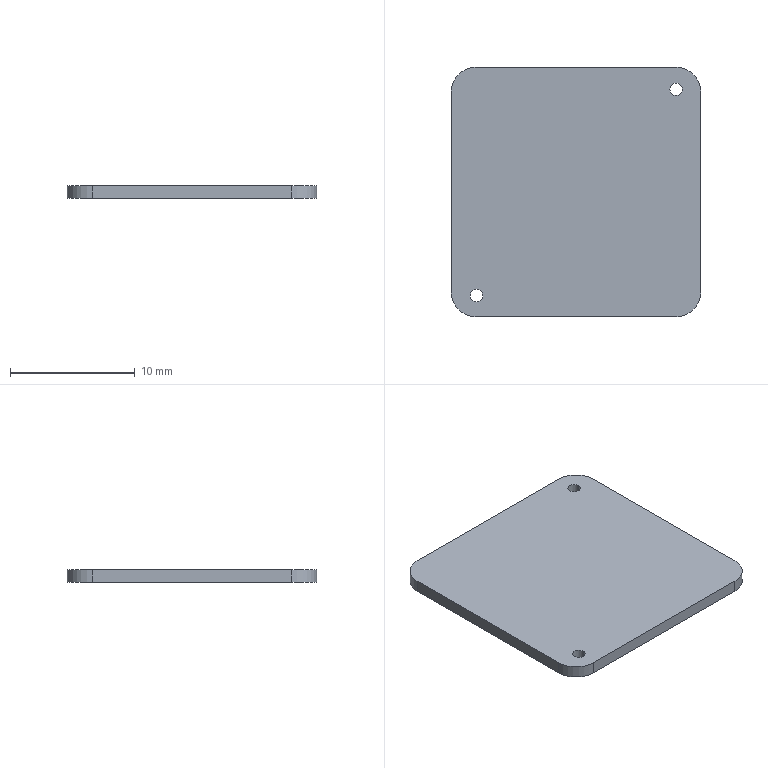Part | SolidWorks | features Extrusion 1, Fillet 1, ICE 1 | 1 solid | 14 faces | box 20 x 20 x 1 mm | volume 394.996 mm3 | cylinder 8 | plane 6 | commonest cylinder face diameters 1 x4 4 x4
STEP:
#1=CARTESIAN_POINT('',(-8.473,-8.297,0.));
#2=VERTEX_POINT('',#1);
#3=CARTESIAN_POINT('',(-7.473,-8.297,0.));
#4=VERTEX_POINT('',#3);
#5=CARTESIAN_POINT('',(-7.973,-8.297,0.));
#6=DIRECTION('',(0.,0.,1.));
#7=DIRECTION('',(1.,0.,0.));
#8=AXIS2_PLACEMENT_3D('',#5,#6,#7);
#9=CIRCLE('',#8,0.5);
#10=EDGE_CURVE('',#2,#4,#9,.T.);
#11=ORIENTED_EDGE('',*,*,#10,.F.);
#12=CARTESIAN_POINT('',(-8.473,-8.297,1.));
#13=VERTEX_POINT('',#12);
#14=CARTESIAN_POINT('',(-8.473,-8.297,0.));
#15=DIRECTION('',(0.,0.,1.));
#16=VECTOR('',#15,1000.);
#17=LINE('',#14,#16);
#18=EDGE_CURVE('',#2,#13,#17,.T.);
#19=ORIENTED_EDGE('',*,*,#18,.T.);
#20=CARTESIAN_POINT('',(-7.473,-8.297,1.));
#21=VERTEX_POINT('',#20);
#22=CARTESIAN_POINT('',(-7.973,-8.297,1.));
#23=DIRECTION('',(0.,0.,1.));
#24=DIRECTION('',(1.,0.,0.));
#25=AXIS2_PLACEMENT_3D('',#22,#23,#24);
#26=CIRCLE('',#25,0.5);
#27=EDGE_CURVE('',#13,#21,#26,.T.);
#28=ORIENTED_EDGE('',*,*,#27,.T.);
#29=CARTESIAN_POINT('',(-7.473,-8.297,0.));
#30=DIRECTION('',(0.,0.,1.));
#31=VECTOR('',#30,1000.);
#32=LINE('',#29,#31);
#33=EDGE_CURVE('',#4,#21,#32,.T.);
#34=ORIENTED_EDGE('',*,*,#33,.F.);
#35=EDGE_LOOP('',(#11,#19,#28,#34));
#36=FACE_OUTER_BOUND('',#35,.T.);
#37=CARTESIAN_POINT('',(-7.973,-8.297,0.));
#38=DIRECTION('',(0.,0.,1.));
#39=DIRECTION('',(1.,0.,0.));
#40=AXIS2_PLACEMENT_3D('',#37,#38,#39);
#41=CYLINDRICAL_SURFACE('',#40,0.5);
#42=ADVANCED_FACE('',(#36),#41,.F.);
#43=CARTESIAN_POINT('',(7.521,8.23,0.));
#44=VERTEX_POINT('',#43);
#45=CARTESIAN_POINT('',(8.521,8.23,0.));
#46=VERTEX_POINT('',#45);
#47=CARTESIAN_POINT('',(8.021,8.23,0.));
#48=DIRECTION('',(0.,0.,1.));
#49=DIRECTION('',(1.,0.,0.));
#50=AXIS2_PLACEMENT_3D('',#47,#48,#49);
#51=CIRCLE('',#50,0.5);
#52=EDGE_CURVE('',#44,#46,#51,.T.);
#53=ORIENTED_EDGE('',*,*,#52,.F.);
#54=CARTESIAN_POINT('',(7.521,8.23,1.));
#55=VERTEX_POINT('',#54);
#56=CARTESIAN_POINT('',(7.521,8.23,0.));
#57=DIRECTION('',(0.,0.,1.));
#58=VECTOR('',#57,1000.);
#59=LINE('',#56,#58);
#60=EDGE_CURVE('',#44,#55,#59,.T.);
#61=ORIENTED_EDGE('',*,*,#60,.T.);
#62=CARTESIAN_POINT('',(8.521,8.23,1.));
#63=VERTEX_POINT('',#62);
#64=CARTESIAN_POINT('',(8.021,8.23,1.));
#65=DIRECTION('',(0.,0.,1.));
#66=DIRECTION('',(1.,0.,0.));
#67=AXIS2_PLACEMENT_3D('',#64,#65,#66);
#68=CIRCLE('',#67,0.5);
#69=EDGE_CURVE('',#55,#63,#68,.T.);
#70=ORIENTED_EDGE('',*,*,#69,.T.);
#71=CARTESIAN_POINT('',(8.521,8.23,0.));
#72=DIRECTION('',(0.,0.,1.));
#73=VECTOR('',#72,1000.);
#74=LINE('',#71,#73);
#75=EDGE_CURVE('',#46,#63,#74,.T.);
#76=ORIENTED_EDGE('',*,*,#75,.F.);
#77=EDGE_LOOP('',(#53,#61,#70,#76));
#78=FACE_OUTER_BOUND('',#77,.T.);
#79=CARTESIAN_POINT('',(8.021,8.23,0.));
#80=DIRECTION('',(0.,0.,1.));
#81=DIRECTION('',(1.,0.,0.));
#82=AXIS2_PLACEMENT_3D('',#79,#80,#81);
#83=CYLINDRICAL_SURFACE('',#82,0.5);
#84=ADVANCED_FACE('',(#78),#83,.F.);
#85=CARTESIAN_POINT('',(10.,-8.,0.));
#86=VERTEX_POINT('',#85);
#87=CARTESIAN_POINT('',(10.,8.,0.));
#88=VERTEX_POINT('',#87);
#89=CARTESIAN_POINT('',(10.,10.,0.));
#90=DIRECTION('',(0.,1.,0.));
#91=VECTOR('',#90,1000.);
#92=LINE('',#89,#91);
#93=EDGE_CURVE('',#86,#88,#92,.T.);
#94=ORIENTED_EDGE('',*,*,#93,.T.);
#95=CARTESIAN_POINT('',(10.,8.,1.));
#96=VERTEX_POINT('',#95);
#97=CARTESIAN_POINT('',(10.,8.,1.));
#98=DIRECTION('',(0.,0.,1.));
#99=VECTOR('',#98,1000.);
#100=LINE('',#97,#99);
#101=EDGE_CURVE('',#88,#96,#100,.T.);
#102=ORIENTED_EDGE('',*,*,#101,.T.);
#103=CARTESIAN_POINT('',(10.,-8.,1.));
#104=VERTEX_POINT('',#103);
#105=CARTESIAN_POINT('',(10.,10.,1.));
#106=DIRECTION('',(0.,1.,0.));
#107=VECTOR('',#106,1000.);
#108=LINE('',#105,#107);
#109=EDGE_CURVE('',#104,#96,#108,.T.);
#110=ORIENTED_EDGE('',*,*,#109,.F.);
#111=CARTESIAN_POINT('',(10.,-8.,1.));
#112=DIRECTION('',(0.,0.,-1.));
#113=VECTOR('',#112,1000.);
#114=LINE('',#111,#113);
#115=EDGE_CURVE('',#104,#86,#114,.T.);
#116=ORIENTED_EDGE('',*,*,#115,.T.);
#117=EDGE_LOOP('',(#94,#102,#110,#116));
#118=FACE_OUTER_BOUND('',#117,.T.);
#119=CARTESIAN_POINT('',(10.,10.,1.));
#120=DIRECTION('',(-1.,0.,0.));
#121=DIRECTION('',(0.,0.,1.));
#122=AXIS2_PLACEMENT_3D('',#119,#120,#121);
#123=PLANE('',#122);
#124=ADVANCED_FACE('',(#118),#123,.F.);
#125=CARTESIAN_POINT('',(8.,10.,1.));
#126=VERTEX_POINT('',#125);
#127=CARTESIAN_POINT('',(-8.,10.,1.));
#128=VERTEX_POINT('',#127);
#129=CARTESIAN_POINT('',(-10.,10.,1.));
#130=DIRECTION('',(-1.,0.,0.));
#131=VECTOR('',#130,1000.);
#132=LINE('',#129,#131);
#133=EDGE_CURVE('',#126,#128,#132,.T.);
#134=ORIENTED_EDGE('',*,*,#133,.F.);
#135=CARTESIAN_POINT('',(8.,10.,0.));
#136=VERTEX_POINT('',#135);
#137=CARTESIAN_POINT('',(8.,10.,1.));
#138=DIRECTION('',(0.,0.,-1.));
#139=VECTOR('',#138,1000.);
#140=LINE('',#137,#139);
#141=EDGE_CURVE('',#126,#136,#140,.T.);
#142=ORIENTED_EDGE('',*,*,#141,.T.);
#143=CARTESIAN_POINT('',(-8.,10.,0.));
#144=VERTEX_POINT('',#143);
#145=CARTESIAN_POINT('',(-10.,10.,0.));
#146=DIRECTION('',(-1.,0.,0.));
#147=VECTOR('',#146,1000.);
#148=LINE('',#145,#147);
#149=EDGE_CURVE('',#136,#144,#148,.T.);
#150=ORIENTED_EDGE('',*,*,#149,.T.);
#151=CARTESIAN_POINT('',(-8.,10.,1.));
#152=DIRECTION('',(0.,0.,1.));
#153=VECTOR('',#152,1000.);
#154=LINE('',#151,#153);
#155=EDGE_CURVE('',#144,#128,#154,.T.);
#156=ORIENTED_EDGE('',*,*,#155,.T.);
#157=EDGE_LOOP('',(#134,#142,#150,#156));
#158=FACE_OUTER_BOUND('',#157,.T.);
#159=CARTESIAN_POINT('',(-10.,10.,1.));
#160=DIRECTION('',(0.,-1.,0.));
#161=DIRECTION('',(0.,0.,-1.));
#162=AXIS2_PLACEMENT_3D('',#159,#160,#161);
#163=PLANE('',#162);
#164=ADVANCED_FACE('',(#158),#163,.F.);
#165=CARTESIAN_POINT('',(-10.,8.,0.));
#166=VERTEX_POINT('',#165);
#167=CARTESIAN_POINT('',(-10.,-8.,0.));
#168=VERTEX_POINT('',#167);
#169=CARTESIAN_POINT('',(-10.,10.,0.));
#170=DIRECTION('',(0.,-1.,0.));
#171=VECTOR('',#170,1000.);
#172=LINE('',#169,#171);
#173=EDGE_CURVE('',#166,#168,#172,.T.);
#174=ORIENTED_EDGE('',*,*,#173,.T.);
#175=CARTESIAN_POINT('',(-10.,-8.,1.));
#176=VERTEX_POINT('',#175);
#177=CARTESIAN_POINT('',(-10.,-8.,1.));
#178=DIRECTION('',(0.,0.,1.));
#179=VECTOR('',#178,1000.);
#180=LINE('',#177,#179);
#181=EDGE_CURVE('',#168,#176,#180,.T.);
#182=ORIENTED_EDGE('',*,*,#181,.T.);
#183=CARTESIAN_POINT('',(-10.,8.,1.));
#184=VERTEX_POINT('',#183);
#185=CARTESIAN_POINT('',(-10.,10.,1.));
#186=DIRECTION('',(0.,-1.,0.));
#187=VECTOR('',#186,1000.);
#188=LINE('',#185,#187);
#189=EDGE_CURVE('',#184,#176,#188,.T.);
#190=ORIENTED_EDGE('',*,*,#189,.F.);
#191=CARTESIAN_POINT('',(-10.,8.,1.));
#192=DIRECTION('',(0.,0.,-1.));
#193=VECTOR('',#192,1000.);
#194=LINE('',#191,#193);
#195=EDGE_CURVE('',#184,#166,#194,.T.);
#196=ORIENTED_EDGE('',*,*,#195,.T.);
#197=EDGE_LOOP('',(#174,#182,#190,#196));
#198=FACE_OUTER_BOUND('',#197,.T.);
#199=CARTESIAN_POINT('',(-10.,10.,1.));
#200=DIRECTION('',(1.,0.,0.));
#201=DIRECTION('',(0.,0.,-1.));
#202=AXIS2_PLACEMENT_3D('',#199,#200,#201);
#203=PLANE('',#202);
#204=ADVANCED_FACE('',(#198),#203,.F.);
#205=CARTESIAN_POINT('',(-8.,-10.,1.));
#206=VERTEX_POINT('',#205);
#207=CARTESIAN_POINT('',(8.,-10.,1.));
#208=VERTEX_POINT('',#207);
#209=CARTESIAN_POINT('',(-10.,-10.,1.));
#210=DIRECTION('',(1.,0.,0.));
#211=VECTOR('',#210,1000.);
#212=LINE('',#209,#211);
#213=EDGE_CURVE('',#206,#208,#212,.T.);
#214=ORIENTED_EDGE('',*,*,#213,.F.);
#215=CARTESIAN_POINT('',(-8.,-10.,0.));
#216=VERTEX_POINT('',#215);
#217=CARTESIAN_POINT('',(-8.,-10.,1.));
#218=DIRECTION('',(0.,0.,-1.));
#219=VECTOR('',#218,1000.);
#220=LINE('',#217,#219);
#221=EDGE_CURVE('',#206,#216,#220,.T.);
#222=ORIENTED_EDGE('',*,*,#221,.T.);
#223=CARTESIAN_POINT('',(8.,-10.,0.));
#224=VERTEX_POINT('',#223);
#225=CARTESIAN_POINT('',(-10.,-10.,0.));
#226=DIRECTION('',(1.,0.,0.));
#227=VECTOR('',#226,1000.);
#228=LINE('',#225,#227);
#229=EDGE_CURVE('',#216,#224,#228,.T.);
#230=ORIENTED_EDGE('',*,*,#229,.T.);
#231=CARTESIAN_POINT('',(8.,-10.,1.));
#232=DIRECTION('',(0.,0.,1.));
#233=VECTOR('',#232,1000.);
#234=LINE('',#231,#233);
#235=EDGE_CURVE('',#224,#208,#234,.T.);
#236=ORIENTED_EDGE('',*,*,#235,.T.);
#237=EDGE_LOOP('',(#214,#222,#230,#236));
#238=FACE_OUTER_BOUND('',#237,.T.);
#239=CARTESIAN_POINT('',(-10.,-10.,1.));
#240=DIRECTION('',(0.,1.,0.));
#241=DIRECTION('',(0.,0.,1.));
#242=AXIS2_PLACEMENT_3D('',#239,#240,#241);
#243=PLANE('',#242);
#244=ADVANCED_FACE('',(#238),#243,.F.);
#245=CARTESIAN_POINT('',(-7.973,-8.297,1.));
#246=DIRECTION('',(0.,0.,1.));
#247=DIRECTION('',(1.,0.,0.));
#248=AXIS2_PLACEMENT_3D('',#245,#246,#247);
#249=CIRCLE('',#248,0.5);
#250=EDGE_CURVE('',#21,#13,#249,.T.);
#251=ORIENTED_EDGE('',*,*,#250,.F.);
#252=ORIENTED_EDGE('',*,*,#27,.F.);
#253=EDGE_LOOP('',(#251,#252));
#254=FACE_BOUND('',#253,.T.);
#255=CARTESIAN_POINT('',(8.021,8.23,1.));
#256=DIRECTION('',(0.,0.,1.));
#257=DIRECTION('',(1.,0.,0.));
#258=AXIS2_PLACEMENT_3D('',#255,#256,#257);
#259=CIRCLE('',#258,0.5);
#260=EDGE_CURVE('',#63,#55,#259,.T.);
#261=ORIENTED_EDGE('',*,*,#260,.F.);
#262=ORIENTED_EDGE('',*,*,#69,.F.);
#263=EDGE_LOOP('',(#261,#262));
#264=FACE_BOUND('',#263,.T.);
#265=ORIENTED_EDGE('',*,*,#109,.T.);
#266=CARTESIAN_POINT('',(8.,8.,1.));
#267=DIRECTION('',(0.,0.,1.));
#268=DIRECTION('',(1.,0.,0.));
#269=AXIS2_PLACEMENT_3D('',#266,#267,#268);
#270=CIRCLE('',#269,2.);
#271=EDGE_CURVE('',#96,#126,#270,.T.);
#272=ORIENTED_EDGE('',*,*,#271,.T.);
#273=ORIENTED_EDGE('',*,*,#133,.T.);
#274=CARTESIAN_POINT('',(-8.,8.,1.));
#275=DIRECTION('',(0.,0.,1.));
#276=DIRECTION('',(1.,0.,0.));
#277=AXIS2_PLACEMENT_3D('',#274,#275,#276);
#278=CIRCLE('',#277,2.);
#279=EDGE_CURVE('',#128,#184,#278,.T.);
#280=ORIENTED_EDGE('',*,*,#279,.T.);
#281=ORIENTED_EDGE('',*,*,#189,.T.);
#282=CARTESIAN_POINT('',(-8.,-8.,1.));
#283=DIRECTION('',(0.,0.,1.));
#284=DIRECTION('',(1.,0.,0.));
#285=AXIS2_PLACEMENT_3D('',#282,#283,#284);
#286=CIRCLE('',#285,2.);
#287=EDGE_CURVE('',#176,#206,#286,.T.);
#288=ORIENTED_EDGE('',*,*,#287,.T.);
#289=ORIENTED_EDGE('',*,*,#213,.T.);
#290=CARTESIAN_POINT('',(8.,-8.,1.));
#291=DIRECTION('',(0.,0.,1.));
#292=DIRECTION('',(1.,0.,0.));
#293=AXIS2_PLACEMENT_3D('',#290,#291,#292);
#294=CIRCLE('',#293,2.);
#295=EDGE_CURVE('',#208,#104,#294,.T.);
#296=ORIENTED_EDGE('',*,*,#295,.T.);
#297=EDGE_LOOP('',(#265,#272,#273,#280,#281,#288,#289,#296));
#298=FACE_OUTER_BOUND('',#297,.T.);
#299=CARTESIAN_POINT('',(0.,0.,1.));
#300=DIRECTION('',(0.,0.,1.));
#301=DIRECTION('',(1.,0.,0.));
#302=AXIS2_PLACEMENT_3D('',#299,#300,#301);
#303=PLANE('',#302);
#304=ADVANCED_FACE('',(#254,#264,#298),#303,.T.);
#305=CARTESIAN_POINT('',(-7.973,-8.297,0.));
#306=DIRECTION('',(0.,0.,1.));
#307=DIRECTION('',(1.,0.,0.));
#308=AXIS2_PLACEMENT_3D('',#305,#306,#307);
#309=CIRCLE('',#308,0.5);
#310=EDGE_CURVE('',#4,#2,#309,.T.);
#311=ORIENTED_EDGE('',*,*,#310,.T.);
#312=ORIENTED_EDGE('',*,*,#10,.T.);
#313=EDGE_LOOP('',(#311,#312));
#314=FACE_BOUND('',#313,.T.);
#315=CARTESIAN_POINT('',(8.021,8.23,0.));
#316=DIRECTION('',(0.,0.,1.));
#317=DIRECTION('',(1.,0.,0.));
#318=AXIS2_PLACEMENT_3D('',#315,#316,#317);
#319=CIRCLE('',#318,0.5);
#320=EDGE_CURVE('',#46,#44,#319,.T.);
#321=ORIENTED_EDGE('',*,*,#320,.T.);
#322=ORIENTED_EDGE('',*,*,#52,.T.);
#323=EDGE_LOOP('',(#321,#322));
#324=FACE_BOUND('',#323,.T.);
#325=ORIENTED_EDGE('',*,*,#149,.F.);
#326=CARTESIAN_POINT('',(8.,8.,0.));
#327=DIRECTION('',(0.,0.,-1.));
#328=DIRECTION('',(1.,0.,0.));
#329=AXIS2_PLACEMENT_3D('',#326,#327,#328);
#330=CIRCLE('',#329,2.);
#331=EDGE_CURVE('',#136,#88,#330,.T.);
#332=ORIENTED_EDGE('',*,*,#331,.T.);
#333=ORIENTED_EDGE('',*,*,#93,.F.);
#334=CARTESIAN_POINT('',(8.,-8.,0.));
#335=DIRECTION('',(0.,0.,-1.));
#336=DIRECTION('',(1.,0.,0.));
#337=AXIS2_PLACEMENT_3D('',#334,#335,#336);
#338=CIRCLE('',#337,2.);
#339=EDGE_CURVE('',#86,#224,#338,.T.);
#340=ORIENTED_EDGE('',*,*,#339,.T.);
#341=ORIENTED_EDGE('',*,*,#229,.F.);
#342=CARTESIAN_POINT('',(-8.,-8.,0.));
#343=DIRECTION('',(0.,0.,-1.));
#344=DIRECTION('',(1.,0.,0.));
#345=AXIS2_PLACEMENT_3D('',#342,#343,#344);
#346=CIRCLE('',#345,2.);
#347=EDGE_CURVE('',#216,#168,#346,.T.);
#348=ORIENTED_EDGE('',*,*,#347,.T.);
#349=ORIENTED_EDGE('',*,*,#173,.F.);
#350=CARTESIAN_POINT('',(-8.,8.,0.));
#351=DIRECTION('',(0.,0.,-1.));
#352=DIRECTION('',(1.,0.,0.));
#353=AXIS2_PLACEMENT_3D('',#350,#351,#352);
#354=CIRCLE('',#353,2.);
#355=EDGE_CURVE('',#166,#144,#354,.T.);
#356=ORIENTED_EDGE('',*,*,#355,.T.);
#357=EDGE_LOOP('',(#325,#332,#333,#340,#341,#348,#349,#356));
#358=FACE_OUTER_BOUND('',#357,.T.);
#359=CARTESIAN_POINT('',(0.,0.,0.));
#360=DIRECTION('',(0.,0.,1.));
#361=DIRECTION('',(1.,0.,0.));
#362=AXIS2_PLACEMENT_3D('',#359,#360,#361);
#363=PLANE('',#362);
#364=ADVANCED_FACE('',(#314,#324,#358),#363,.F.);
#365=ORIENTED_EDGE('',*,*,#60,.F.);
#366=ORIENTED_EDGE('',*,*,#320,.F.);
#367=ORIENTED_EDGE('',*,*,#75,.T.);
#368=ORIENTED_EDGE('',*,*,#260,.T.);
#369=EDGE_LOOP('',(#365,#366,#367,#368));
#370=FACE_OUTER_BOUND('',#369,.T.);
#371=CARTESIAN_POINT('',(8.021,8.23,0.));
#372=DIRECTION('',(0.,0.,1.));
#373=DIRECTION('',(1.,0.,0.));
#374=AXIS2_PLACEMENT_3D('',#371,#372,#373);
#375=CYLINDRICAL_SURFACE('',#374,0.5);
#376=ADVANCED_FACE('',(#370),#375,.F.);
#377=ORIENTED_EDGE('',*,*,#18,.F.);
#378=ORIENTED_EDGE('',*,*,#310,.F.);
#379=ORIENTED_EDGE('',*,*,#33,.T.);
#380=ORIENTED_EDGE('',*,*,#250,.T.);
#381=EDGE_LOOP('',(#377,#378,#379,#380));
#382=FACE_OUTER_BOUND('',#381,.T.);
#383=CARTESIAN_POINT('',(-7.973,-8.297,0.));
#384=DIRECTION('',(0.,0.,1.));
#385=DIRECTION('',(1.,0.,0.));
#386=AXIS2_PLACEMENT_3D('',#383,#384,#385);
#387=CYLINDRICAL_SURFACE('',#386,0.5);
#388=ADVANCED_FACE('',(#382),#387,.F.);
#389=ORIENTED_EDGE('',*,*,#271,.F.);
#390=ORIENTED_EDGE('',*,*,#101,.F.);
#391=ORIENTED_EDGE('',*,*,#331,.F.);
#392=ORIENTED_EDGE('',*,*,#141,.F.);
#393=EDGE_LOOP('',(#389,#390,#391,#392));
#394=FACE_OUTER_BOUND('',#393,.T.);
#395=CARTESIAN_POINT('',(8.,8.,1.));
#396=DIRECTION('',(0.,0.,-1.));
#397=DIRECTION('',(-1.,0.,0.));
#398=AXIS2_PLACEMENT_3D('',#395,#396,#397);
#399=CYLINDRICAL_SURFACE('',#398,2.);
#400=ADVANCED_FACE('',(#394),#399,.T.);
#401=ORIENTED_EDGE('',*,*,#287,.F.);
#402=ORIENTED_EDGE('',*,*,#181,.F.);
#403=ORIENTED_EDGE('',*,*,#347,.F.);
#404=ORIENTED_EDGE('',*,*,#221,.F.);
#405=EDGE_LOOP('',(#401,#402,#403,#404));
#406=FACE_OUTER_BOUND('',#405,.T.);
#407=CARTESIAN_POINT('',(-8.,-8.,1.));
#408=DIRECTION('',(0.,0.,-1.));
#409=DIRECTION('',(-1.,0.,0.));
#410=AXIS2_PLACEMENT_3D('',#407,#408,#409);
#411=CYLINDRICAL_SURFACE('',#410,2.);
#412=ADVANCED_FACE('',(#406),#411,.T.);
#413=ORIENTED_EDGE('',*,*,#295,.F.);
#414=ORIENTED_EDGE('',*,*,#235,.F.);
#415=ORIENTED_EDGE('',*,*,#339,.F.);
#416=ORIENTED_EDGE('',*,*,#115,.F.);
#417=EDGE_LOOP('',(#413,#414,#415,#416));
#418=FACE_OUTER_BOUND('',#417,.T.);
#419=CARTESIAN_POINT('',(8.,-8.,1.));
#420=DIRECTION('',(0.,0.,-1.));
#421=DIRECTION('',(-1.,0.,0.));
#422=AXIS2_PLACEMENT_3D('',#419,#420,#421);
#423=CYLINDRICAL_SURFACE('',#422,2.);
#424=ADVANCED_FACE('',(#418),#423,.T.);
#425=ORIENTED_EDGE('',*,*,#279,.F.);
#426=ORIENTED_EDGE('',*,*,#155,.F.);
#427=ORIENTED_EDGE('',*,*,#355,.F.);
#428=ORIENTED_EDGE('',*,*,#195,.F.);
#429=EDGE_LOOP('',(#425,#426,#427,#428));
#430=FACE_OUTER_BOUND('',#429,.T.);
#431=CARTESIAN_POINT('',(-8.,8.,1.));
#432=DIRECTION('',(0.,0.,-1.));
#433=DIRECTION('',(-1.,0.,0.));
#434=AXIS2_PLACEMENT_3D('',#431,#432,#433);
#435=CYLINDRICAL_SURFACE('',#434,2.);
#436=ADVANCED_FACE('',(#430),#435,.T.);
#437=CLOSED_SHELL('',(#42,#84,#124,#164,#204,#244,#304,#364,#376,#388,#400,#412,#424,#436));
#438=MANIFOLD_SOLID_BREP('',#437);
#439=CARTESIAN_POINT('',(0.,0.,0.));
#440=DIRECTION('',(0.,0.,1.));
#441=DIRECTION('',(1.,0.,0.));
#442=AXIS2_PLACEMENT_3D('',#439,#440,#441);
#443=(LENGTH_UNIT()NAMED_UNIT(*)SI_UNIT(.MILLI.,.METRE.));
#444=UNCERTAINTY_MEASURE_WITH_UNIT(LENGTH_MEASURE(0.00001),#443,'','');
#445=(NAMED_UNIT(*)PLANE_ANGLE_UNIT()SI_UNIT($,.RADIAN.));
#446=(NAMED_UNIT(*)SI_UNIT($,.STERADIAN.)SOLID_ANGLE_UNIT());
#447=(GEOMETRIC_REPRESENTATION_CONTEXT(3)GLOBAL_UNCERTAINTY_ASSIGNED_CONTEXT((#444))GLOBAL_UNIT_ASSIGNED_CONTEXT((#443,#445,#446))REPRESENTATION_CONTEXT('',''));
#448=ADVANCED_BREP_SHAPE_REPRESENTATION('',(#438,#442),#447);